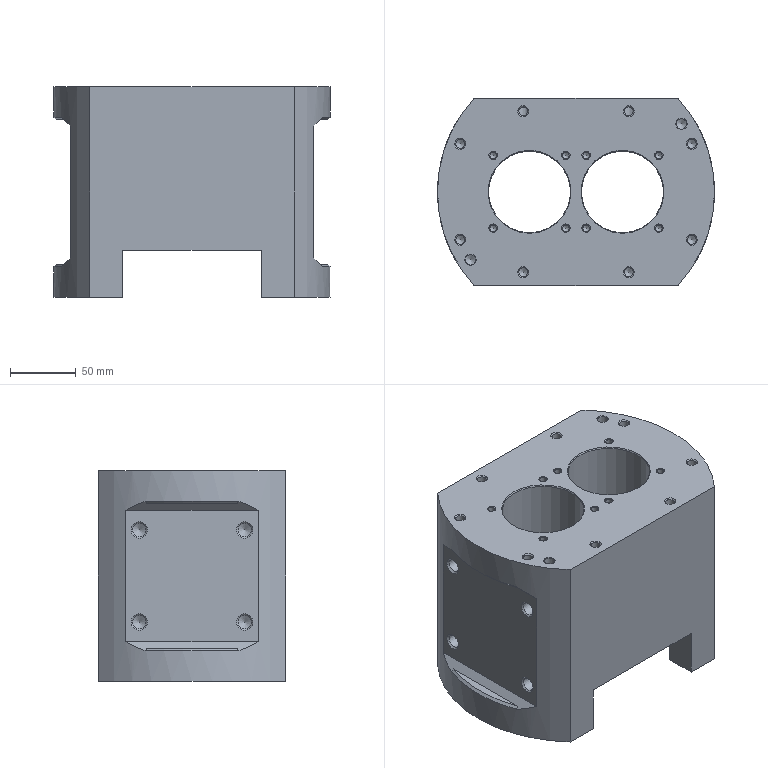NC program | NX | posted with a generic post | part box 210 x 142 x 160 mm
Whole program:
N10 G17 G21 G94 G90
(FLOOR_WALL_COPY_1 , TOOL : D50)
N12 T02 M6
N14 G54
N16 G17 G0 G90 X46.563 Y-89.997 B0. C0. S1200 M3
N18 G43 Z30. H2
N20 Z2.65
N22 G94 G1 Z-0.35 F1000.
N24 X43.563
N26 X-43.563 F2000.
N28 Y-49.998
N30 X43.563
N32 Y-9.999
N34 X-43.563
N36 Y30.001
N38 X43.563
N40 Y70.
N42 X-43.563
N44 X-46.563
N46 Z2.65
N48 G0 Z30.
N50 X50.098 Y-89.997
N52 Z2.301
N54 G1 Z-0.699 F1000.
N56 X47.098
N58 X-47.098 F2000.
N60 Y-49.998
N62 X47.098
N64 Y-9.999
N66 X-47.098
N68 Y30.001
N70 X47.098
N72 Y70.
N74 X-47.098
N76 X-50.098
N78 Z2.301
N80 G0 Z30.
N82 X52.803 Y-89.997
N84 Z1.951
N86 G1 Z-1.049 F1000.
N88 X49.803
N90 X-49.803 F2000.
N92 Y-49.998
N94 X49.803
N96 Y-9.999
N98 X-49.803
N100 Y30.001
N102 X49.803
N104 Y70.
N106 X-49.803
N108 X-52.803
N110 Z1.951
N112 G0 Z30.
N114 X55.078 Y-89.997
N116 Z1.602
N118 G1 Z-1.398 F1000.
N120 X52.078
N122 X-52.078 F2000.
N124 Y-49.998
N126 X52.078
N128 Y-9.999
N130 X-52.078
N132 Y30.001
N134 X52.078
N136 Y70.
N138 X-52.078
N140 X-55.078
N142 Z1.602
N144 G0 Z30.
N146 X57.078 Y-89.997
N148 Z1.252
N150 G1 Z-1.748 F1000.
N152 X54.078
N154 X-54.078 F2000.
N156 Y-49.998
N158 X54.078
N160 Y-9.999
N162 X-54.078
N164 Y30.001
N166 X54.078
N168 Y70.
N170 X-54.078
N172 X-57.078
N174 Z1.252
N176 G0 Z30.
N178 X58.881 Y-89.997
N180 Z0.903
N182 G1 Z-2.097 F1000.
N184 X55.881
N186 X-55.881 F2000.
N188 Y-49.998
N190 X55.881
N192 Y-9.999
N194 X-55.881
N196 Y30.001
N198 X55.881
N200 Y70.
N202 X-55.881
N204 X-58.881
N206 Z0.903
N208 G0 Z30.
N210 X60.535 Y-89.997
N212 Z0.553
N214 G1 Z-2.447 F1000.
N216 X57.535
N218 X-57.535 F2000.
N220 Y-49.998
N222 X57.535
N224 Y-9.999
N226 X-57.535
N228 Y30.001
N230 X57.535
N232 Y70.
N234 X-57.535
N236 X-60.535
N238 Z0.553
N240 G0 Z30.
N242 X62.07 Y-89.997
N244 Z0.204
N246 G1 Z-2.796 F1000.
N248 X59.07
N250 X-59.07 F2000.
N252 Y-49.998
N254 X59.07
N256 Y-9.999
N258 X-59.07
N260 Y30.001
N262 X59.07
N264 Y70.
N266 X-59.07
N268 X-62.07
N270 Z0.204
N272 G0 Z30.
N274 X63.509 Y-89.997
N276 Z-0.146
N278 G1 Z-3.146 F1000.
N280 X60.509
N282 X-60.509 F2000.
N284 Y-49.998
N286 X60.509
N288 Y-9.999
N290 X-60.509
N292 Y30.001
N294 X60.509
N296 Y70.
N298 X-60.509
N300 X-63.509
N302 Z-0.146
N304 G0 Z30.
N306 X64.866 Y-89.997
N308 Z-0.495
N310 G1 Z-3.495 F1000.
N312 X61.866
N314 X-61.866 F2000.
N316 Y-49.998
N318 X61.866
N320 Y-9.999
N322 X-61.866
N324 Y30.001
N326 X61.866
N328 Y70.
N330 X-61.866
N332 X-64.866
N334 Z-0.495
N336 G0 Z30.
N338 X66.153 Y-89.997
N340 Z-0.845
N342 G1 Z-3.845 F1000.
N344 X63.153
N346 X-63.153 F2000.
N348 Y-49.998
N350 X63.153
N352 Y-9.999
N354 X-63.153
N356 Y30.001
N358 X63.153
N360 Y70.
N362 X-63.153
N364 X-66.153
N366 Z-0.845
N368 G0 Z30.
N370 X67.38 Y-89.997
N372 Z-1.194
N374 G1 Z-4.194 F1000.
N376 X64.38
N378 X-64.38 F2000.
N380 Y-49.998
N382 X64.38
N384 Y-9.999
N386 X-64.38
N388 Y30.001
N390 X64.38
N392 Y70.
N394 X-64.38
N396 X-67.38
N398 Z-1.194
N400 G0 Z30.
N402 X68.553 Y-89.997
N404 Z-1.544
N406 G1 Z-4.544 F1000.
N408 X65.553
N410 X-65.553 F2000.
N412 Y-49.998
N414 X65.553
N416 Y-9.999
N418 X-65.553
N420 Y30.001
N422 X65.553
N424 Y70.
N426 X-65.553
N428 X-68.553
N430 Z-1.544
N432 G0 Z30.
N434 X69.68 Y-89.997
N436 Z-1.893
N438 G1 Z-4.893 F1000.
N440 X66.68
N442 X-66.68 F2000.
N444 Y-49.998
N446 X66.68
N448 Y-9.999
N450 X-66.68
N452 Y30.001
N454 X66.68
N456 Y70.
N458 X-66.68
N460 X-69.68
N462 Z-1.893
N464 G0 Z30.
N466 X70.763 Y-89.997
N468 Z-2.243
N470 G1 Z-5.243 F1000.
N472 X67.763
N474 X-67.763 F2000.
N476 Y-49.998
N478 X67.763
N480 Y-9.999
N482 X-67.763
N484 Y30.001
N486 X67.763
N488 Y70.
N490 X-67.763
N492 X-70.763
N494 Z-2.243
N496 G0 Z30.
N498 X71.809 Y-89.997
N500 Z-2.592
N502 G1 Z-5.592 F1000.
N504 X68.809
N506 X-68.809 F2000.
N508 Y-49.998
N510 X68.809
N512 Y-9.999
N514 X-68.809
N516 Y30.001
N518 X68.809
N520 Y70.
N522 X-68.809
N524 X-71.809
N526 Z-2.592
N528 G0 Z30.
N530 X72.82 Y-89.997
N532 Z-2.941
N534 G1 Z-5.941 F1000.
N536 X69.82
N538 X-69.82 F2000.
N540 Y-49.998
N542 X69.82
N544 Y-9.999
N546 X-69.82
N548 Y30.001
N550 X69.82
N552 Y70.
N554 X-69.82
N556 X-72.82
N558 Z-2.941
N560 G0 Z30.
N562 X73.798 Y-89.997
N564 Z-3.291
N566 G1 Z-6.291 F1000.
N568 X70.798
N570 X-70.798 F2000.
N572 Y-49.998
N574 X70.798
N576 Y-9.999
N578 X-70.798
N580 Y30.001
N582 X70.798
N584 Y70.
N586 X-70.798
N588 X-73.798
N590 Z-3.291
N592 G0 Z30.
N594 X74.748 Y-89.997
N596 Z-3.64
N598 G1 Z-6.64 F1000.
N600 X71.748
N602 X-71.748 F2000.
N604 Y-49.998
N606 X71.748
N608 Y-9.999
N610 X-71.748
N612 Y30.001
N614 X71.748
N616 Y70.
N618 X-71.748
N620 X-74.748
N622 Z-3.64
N624 G0 Z30.
N626 X75.67 Y-89.997
N628 Z-3.99
N630 G1 Z-6.99 F1000.
N632 X72.67
N634 X-72.67 F2000.
N636 Y-49.998
N638 X72.67
N640 Y-9.999
N642 X-72.67
N644 Y30.001
N646 X72.67
N648 Y70.
N650 X-72.67
N652 X-75.67
N654 Z-3.99
N656 G0 Z30.
N658 X76.567 Y-89.997
N660 Z-4.339
N662 G1 Z-7.339 F1000.
N664 X73.567
N666 X-73.567 F2000.
N668 Y-49.998
N670 X73.567
N672 Y-9.999
N674 X-73.567
N676 Y30.001
N678 X73.567
N680 Y70.
N682 X-73.567
N684 X-76.567
N686 Z-4.339
N688 G0 Z30.
N690 X77.44 Y-89.997
N692 Z-4.689
N694 G1 Z-7.689 F1000.
N696 X74.44
N698 X-74.44 F2000.
N700 Y-49.998
N702 X74.44
N704 Y-9.999
N706 X-74.44
N708 Y30.001
N710 X74.44
N712 Y70.
N714 X-74.44
N716 X-77.44
N718 Z-4.689
N720 G0 Z30.
N722 X78.292 Y-89.997
N724 Z-5.038
N726 G1 Z-8.038 F1000.
N728 X75.292
N730 X-75.292 F2000.
N732 Y-49.998
N734 X75.292
N736 Y-9.999
N738 X-75.292
N740 Y30.001
N742 X75.292
N744 Y70.
N746 X-75.292
N748 X-78.292
N750 Z-5.038
N752 G0 Z30.
N754 X79.123 Y-89.997
N756 Z-5.388
N758 G1 Z-8.388 F1000.
N760 X76.123
N762 X-76.123 F2000.
N764 Y-49.998
N766 X76.123
N768 Y-9.999
N770 X-76.123
N772 Y30.001
N774 X76.123
N776 Y70.
N778 X-76.123
N780 X-79.123
N782 Z-5.388
N784 G0 Z30.
N786 X79.934 Y-89.997
N788 Z-5.737
N790 G1 Z-8.737 F1000.
N792 X76.934
N794 X-76.934 F2000.
N796 Y-49.998
N798 X76.934
N800 Y-9.999
N802 X-76.934
N804 Y30.001
N806 X76.934
N808 Y70.
N810 X-76.934
N812 X-79.934
N814 Z-5.737
N816 G0 Z30.
N818 X80.728 Y-89.997
N820 Z-6.087
N822 G1 Z-9.087 F1000.
N824 X77.728
N826 X-77.728 F2000.
N828 Y-49.998
N830 X77.728
N832 Y-9.999
N834 X-77.728
N836 Y30.001
N838 X77.728
N840 Y70.
N842 X-77.728
N844 X-80.728
N846 Z-6.087
N848 G0 Z30.
N850 X81.504 Y-89.997
N852 Z-6.436
N854 G1 Z-9.436 F1000.
N856 X78.504
N858 X-78.504 F2000.
N860 Y-49.998
N862 X78.504
N864 Y-9.999
N866 X-78.504
N868 Y30.001
N870 X78.504
N872 Y70.
N874 X-78.504
N876 X-81.504
N878 Z-6.436
N880 G0 Z30.
N882 X82.263 Y-89.997
N884 Z-6.786
N886 G1 Z-9.786 F1000.
N888 X79.263
N890 X-79.263 F2000.
N892 Y-49.998
N894 X79.263
N896 Y-9.999
N898 X-79.263
N900 Y30.001
N902 X79.263
N904 Y70.
N906 X-79.263
N908 X-82.263
N910 Z-6.786
N912 G0 Z30.
N914 X83.008 Y-89.997
N916 Z-7.135
N918 G1 Z-10.135 F1000.
N920 X80.008
N922 X-80.008 F2000.
N924 Y-49.998
N926 X80.008
N928 Y-9.999
N930 X-80.008
N932 Y30.001
N934 X80.008
N936 Y70.
N938 X-80.008
N940 X-83.008
N942 Z-7.135
N944 G0 Z30.
N946 X83.737 Y-89.997
N948 Z-7.485
N950 G1 Z-10.485 F1000.
N952 X80.737
N954 X-80.737 F2000.
N956 Y-49.998
N958 X80.737
N960 Y-9.999
N962 X-80.737
N964 Y30.001
N966 X80.737
N968 Y70.
N970 X-80.737
N972 X-83.737
N974 Z-7.485
N976 G0 Z30.
N978 X84.452 Y-89.997
N980 Z-7.834
N982 G1 Z-10.834 F1000.
N984 X81.452
N986 X-81.452 F2000.
N988 Y-49.998
N990 X81.452
N992 Y-9.999
N994 X-81.452
N996 Y30.001
N998 X81.452
N1000 Y70.
N1002 X-81.452
N1004 X-84.452
N1006 Z-7.834
N1008 G0 Z30.
N1010 X85.154 Y-89.997
N1012 Z-8.184
N1014 G1 Z-11.184 F1000.
N1016 X82.154
N1018 X-82.154 F2000.
N1020 Y-49.998
N1022 X82.154
N1024 Y-9.999
N1026 X-82.154
N1028 Y30.001
N1030 X82.154
N1032 Y70.
N1034 X-82.154
N1036 X-85.154
N1038 Z-8.184
N1040 G0 Z30.
N1042 X85.843 Y-89.997
N1044 Z-8.533
N1046 G1 Z-11.533 F1000.
N1048 X82.843
N1050 X-82.843 F2000.
N1052 Y-49.998
N1054 X82.843
N1056 Y-9.999
N1058 X-82.843
N1060 Y30.001
N1062 X82.843
N1064 Y70.
N1066 X-82.843
N1068 X-85.843
N1070 Z-8.533
N1072 G0 Z30.
N1074 X86.52 Y-89.997
N1076 Z-8.883
N1078 G1 Z-11.883 F1000.
N1080 X83.52
N1082 X-83.52 F2000.
N1084 Y-49.998
N1086 X83.52
N1088 Y-9.999
N1090 X-83.52
N1092 Y30.001
N1094 X83.52
N1096 Y70.
N1098 X-83.52
N1100 X-86.52
N1102 Z-8.883
N1104 G0 Z30.
N1106 X87.185 Y-89.997
N1108 Z-9.232
N1110 G1 Z-12.232 F1000.
N1112 X84.185
N1114 X-84.185 F2000.
N1116 Y-49.998
N1118 X84.185
N1120 Y-9.999
N1122 X-84.185
N1124 Y30.001
N1126 X84.185
N1128 Y70.
N1130 X-84.185
N1132 X-87.185
N1134 Z-9.232
N1136 G0 Z30.
N1138 X87.838 Y-89.997
N1140 Z-9.582
N1142 G1 Z-12.582 F1000.
N1144 X84.838
N1146 X-84.838 F2000.
N1148 Y-49.998
N1150 X84.838
N1152 Y-9.999
N1154 X-84.838
N1156 Y30.001
N1158 X84.838
N1160 Y70.
N1162 X-84.838
N1164 X-87.838
N1166 Z-9.582
N1168 G0 Z30.
N1170 X88.481 Y-89.997
N1172 Z-9.931
N1174 G1 Z-12.931 F1000.
N1176 X85.481
N1178 X-85.481 F2000.
N1180 Y-49.998
N1182 X85.481
N1184 Y-9.999
N1186 X-85.481
N1188 Y30.001
N1190 X85.481
N1192 Y70.
N1194 X-85.481
N1196 X-88.481
N1198 Z-9.931
N1200 G0 Z30.
N1202 X89.113 Y-89.997
N1204 Z-10.281
N1206 G1 Z-13.281 F1000.
N1208 X86.113
N1210 X-86.113 F2000.
N1212 Y-49.998
N1214 X86.113
N1216 Y-9.999
N1218 X-86.113
N1220 Y30.001
N1222 X86.113
N1224 Y70.
N1226 X-86.113
N1228 X-89.113
N1230 Z-10.281
N1232 G0 Z30.
N1234 X89.735 Y-89.997
N1236 Z-10.63
N1238 G1 Z-13.63 F1000.
N1240 X86.735
N1242 X-86.735 F2000.
N1244 Y-49.998
N1246 X86.735
N1248 Y-9.999
N1250 X-86.735
N1252 Y30.001
N1254 X86.735
N1256 Y70.
N1258 X-86.735
N1260 X-89.735
N1262 Z-10.63
N1264 G0 Z30.
N1266 X90.348 Y-89.997
N1268 Z-10.98
N1270 G1 Z-13.98 F1000.
N1272 X87.348
N1274 X-87.348 F2000.
N1276 Y-49.998
N1278 X87.348
N1280 Y-9.999
N1282 X-87.348
N1284 Y30.001
N1286 X87.348
N1288 Y70.
N1290 X-87.348
N1292 X-90.348
N1294 Z-10.98
N1296 G0 Z30.
N1298 X90.951 Y-89.997
N1300 Z-11.329
N1302 G1 Z-14.329 F1000.
N1304 X87.951
N1306 X-87.951 F2000.
N1308 Y-49.998
N1310 X87.951
N1312 Y-9.999
N1314 X-87.951
N1316 Y30.001
N1318 X87.951
N1320 Y70.
N1322 X-87.951
N1324 X-90.951
N1326 Z-11.329
N1328 G0 Z30.
N1330 X91.545 Y-89.997
N1332 Z-11.679
N1334 G1 Z-14.679 F1000.
N1336 X88.545
N1338 X-88.545 F2000.
N1340 Y-49.998
N1342 X88.545
N1344 Y-9.999
N1346 X-88.545
N1348 Y30.001
N1350 X88.545
N1352 Y70.
N1354 X-88.545
N1356 X-91.545
N1358 Z-11.679
N1360 G0 Z30.
N1362 X92.13 Y-89.997
N1364 Z-12.028
N1366 G1 Z-15.028 F1000.
N1368 X89.13
N1370 X-89.13 F2000.
N1372 Y-49.998
N1374 X89.13
N1376 Y-9.999
N1378 X-89.13
N1380 Y30.001
N1382 X89.13
N1384 Y70.
N1386 X-89.13
N1388 X-92.13
N1390 Z-12.028
N1392 G0 Z30.
N1394 X92.707 Y-89.997
N1396 Z-12.377
N1398 G1 Z-15.377 F1000.
N1400 X89.707
N1402 X-89.707 F2000.
N1404 Y-49.998
N1406 X89.707
N1408 Y-9.999
N1410 X-89.707
N1412 Y30.001
N1414 X89.707
N1416 Y70.
N1418 X-89.707
N1420 X-92.707
N1422 Z-12.377
N1424 G0 Z30.
N1426 X93.275 Y-89.997
N1428 Z-12.727
N1430 G1 Z-15.727 F1000.
N1432 X90.275
N1434 X-90.275 F2000.
N1436 Y-49.998
N1438 X90.275
N1440 Y-9.999
N1442 X-90.275
N1444 Y30.001
N1446 X90.275
N1448 Y70.
N1450 X-90.275
N1452 X-93.275
N1454 Z-12.727
N1456 G0 Z30.
N1458 X93.835 Y-89.997
N1460 Z-13.076
N1462 G1 Z-16.076 F1000.
N1464 X90.835
N1466 X-90.835 F2000.
N1468 Y-49.998
N1470 X90.835
N1472 Y-9.999
N1474 X-90.835
N1476 Y30.001
N1478 X90.835
N1480 Y70.
N1482 X-90.835
N1484 X-93.835
N1486 Z-13.076
N1488 G0 Z30.
N1490 X94.388 Y-89.997
N1492 Z-13.426
N1494 G1 Z-16.426 F1000.
N1496 X91.388
N1498 X-91.388 F2000.
N1500 Y-49.998
N1502 X91.388
N1504 Y-9.999
N1506 X-91.388
N1508 Y30.001
N1510 X91.388
N1512 Y70.
N1514 X-91.388
N1516 X-94.388
N1518 Z-13.426
N1520 G0 Z30.
N1522 X94.933 Y-89.997
N1524 Z-13.775
N1526 G1 Z-16.775 F1000.
N1528 X91.933
N1530 X-91.933 F2000.
N1532 Y-49.998
N1534 X91.933
N1536 Y-9.999
N1538 X-91.933
N1540 Y30.001
N1542 X91.933
N1544 Y70.
N1546 X-91.933
N1548 X-94.933
N1550 Z-13.775
N1552 G0 Z30.
N1554 X95.471 Y-89.997
N1556 Z-14.125
N1558 G1 Z-17.125 F1000.
N1560 X92.471
N1562 X-92.471 F2000.
N1564 Y-49.998
N1566 X92.471
N1568 Y-9.999
N1570 X-92.471
N1572 Y30.001
N1574 X92.471
N1576 Y70.
N1578 X-92.471
N1580 X-95.471
N1582 Z-14.125
N1584 G0 Z30.
N1586 X96.002 Y-89.997
N1588 Z-14.474
N1590 G1 Z-17.474 F1000.
N1592 X93.002
N1594 X-93.002 F2000.
N1596 Y-49.998
N1598 X93.002
N1600 Y-9.999
N1602 X-93.002
N1604 Y30.001
N1606 X93.002
N1608 Y70.
N1610 X-93.002
N1612 X-96.002
N1614 Z-14.474
N1616 G0 Z30.
N1618 X96.526 Y-89.997
N1620 Z-14.824
N1622 G1 Z-17.824 F1000.
N1624 X93.526
N1626 X-93.526 F2000.
N1628 Y-49.998
N1630 X93.526
N1632 Y-9.999
N1634 X-93.526
N1636 Y30.001
N1638 X93.526
N1640 Y70.
N1642 X-93.526
N1644 X-96.526
N1646 Z-14.824
N1648 G0 Z30.
N1650 X97.043 Y-89.997
N1652 Z-15.173
N1654 G1 Z-18.173 F1000.
N1656 X94.043
N1658 X-94.043 F2000.
N1660 Y-49.998
N1662 X94.043
N1664 Y-9.999
N1666 X-94.043
N1668 Y30.001
N1670 X94.043
N1672 Y70.
N1674 X-94.043
N1676 X-97.043
N1678 Z-15.173
N1680 G0 Z30.
N1682 X97.554 Y-89.997
N1684 Z-15.523
N1686 G1 Z-18.523 F1000.
N1688 X94.554
N1690 X-94.554 F2000.
N1692 Y-49.998
N1694 X94.554
N1696 Y-9.999
N1698 X-94.554
N1700 Y30.001
N1702 X94.554
N1704 Y70.
N1706 X-94.554
N1708 X-97.554
N1710 Z-15.523
N1712 G0 Z30.
N1714 X98.058 Y-89.997
N1716 Z-15.872
N1718 G1 Z-18.872 F1000.
N1720 X95.058
N1722 X-95.058 F2000.
N1724 Y-49.998
N1726 X95.058
N1728 Y-9.999
N1730 X-95.058
N1732 Y30.001
N1734 X95.058
N1736 Y70.
N1738 X-95.058
N1740 X-98.058
N1742 Z-15.872
N1744 G0 Z30.
N1746 X98.557 Y-89.997
N1748 Z-16.222
N1750 G1 Z-19.222 F1000.
N1752 X95.557
N1754 X-95.557 F2000.
N1756 Y-49.998
N1758 X95.557
N1760 Y-9.999
N1762 X-95.557
N1764 Y30.001
N1766 X95.557
N1768 Y70.
N1770 X-95.557
N1772 X-98.557
N1774 Z-16.222
N1776 G0 Z30.
N1778 X99.049 Y-89.997
N1780 Z-16.571
N1782 G1 Z-19.571 F1000.
N1784 X96.049
N1786 X-96.049 F2000.
N1788 Y-49.998
N1790 X96.049
N1792 Y-9.999
N1794 X-96.049
N1796 Y30.001
N1798 X96.049
N1800 Y70.
N1802 X-96.049
N1804 X-99.049
N1806 Z-16.571
N1808 G0 Z30.
N1810 X99.535 Y-89.997
N1812 Z-16.921
N1814 G1 Z-19.921 F1000.
N1816 X96.535
N1818 X-96.535 F2000.
N1820 Y-49.998
N1822 X96.535
N1824 Y-9.999
N1826 X-96.535
N1828 Y30.001
N1830 X96.535
N1832 Y70.
N1834 X-96.535
N1836 X-99.535
N1838 Z-16.921
N1840 G0 Z30.
N1842 X100.015 Y-89.997
N1844 Z-17.27
N1846 G1 Z-20.27 F1000.
N1848 X97.015
N1850 X-97.015 F2000.
N1852 Y-49.998
N1854 X97.015
N1856 Y-9.999
N1858 X-97.015
N1860 Y30.001
N1862 X97.015
N1864 Y70.
N1866 X-97.015
N1868 X-100.015
N1870 Z-17.27
N1872 G0 Z30.
N1874 X100.49 Y-89.997
N1876 Z-17.62
N1878 G1 Z-20.62 F1000.
N1880 X97.49
N1882 X-97.49 F2000.
N1884 Y-49.998
N1886 X97.49
N1888 Y-9.999
N1890 X-97.49
N1892 Y30.001
N1894 X97.49
N1896 Y70.
N1898 X-97.49
N1900 X-100.49
N1902 Z-17.62
N1904 G0 Z30.
N1906 X100.959 Y-89.997
N1908 Z-17.969
N1910 G1 Z-20.969 F1000.
N1912 X97.959
N1914 X-97.959 F2000.
N1916 Y-49.998
N1918 X97.959
N1920 Y-9.999
N1922 X-97.959
N1924 Y30.001
N1926 X97.959
N1928 Y70.
N1930 X-97.959
N1932 X-100.959
N1934 Z-17.969
N1936 G0 Z30.
N1938 X101.423 Y-89.997
N1940 Z-18.319
N1942 G1 Z-21.319 F1000.
N1944 X98.423
N1946 X-98.423 F2000.
N1948 Y-49.998
N1950 X98.423
N1952 Y-9.999
N1954 X-98.423
N1956 Y30.001
N1958 X98.423
N1960 Y70.
N1962 X-98.423
N1964 X-101.423
N1966 Z-18.319
N1968 G0 Z30.
N1970 X101.881 Y-89.997
N1972 Z-18.668
N1974 G1 Z-21.668 F1000.
N1976 X98.881
N1978 X-98.881 F2000.
N1980 Y-49.998
N1982 X98.881
N1984 Y-9.999
N1986 X-98.881
N1988 Y30.001
N1990 X98.881
N1992 Y70.
N1994 X-98.881
N1996 X-101.881
N1998 Z-18.668
N2000 G0 Z30.
N2002 X102.334 Y-89.997
N2004 Z-19.018
N2006 G1 Z-22.018 F1000.
N2008 X99.334
N2010 X-99.334 F2000.
N2012 Y-49.998
N2014 X99.334
N2016 Y-9.999
N2018 X-99.334
N2020 Y30.001
N2022 X99.334
N2024 Y70.
N2026 X-99.334
N2028 X-102.334
N2030 Z-19.018
N2032 G0 Z30.
N2034 X102.783 Y-89.997
N2036 Z-19.367
N2038 G1 Z-22.367 F1000.
N2040 X99.783
N2042 X-99.783 F2000.
N2044 Y-49.998
N2046 X99.783
N2048 Y-9.999
N2050 X-99.783
N2052 Y30.001
N2054 X99.783
N2056 Y70.
N2058 X-99.783
N2060 X-102.783
N2062 Z-19.367
N2064 G0 Z30.
N2066 X103.226 Y-89.997
N2068 Z-19.717
N2070 G1 Z-22.717 F1000.
N2072 X100.226
N2074 X-100.226 F2000.
N2076 Y-49.998
N2078 X100.226
N2080 Y-9.999
N2082 X-100.226
N2084 Y30.001
N2086 X100.226
N2088 Y70.
N2090 X-100.226
N2092 X-103.226
N2094 Z-19.717
N2096 G0 Z30.
N2098 X103.665 Y-89.997
N2100 Z-20.066
N2102 G1 Z-23.066 F1000.
N2104 X100.665
N2106 X-100.665 F2000.
N2108 Y-49.998
N2110 X100.665
N2112 Y-9.999
N2114 X-100.665
N2116 Y30.001
N2118 X100.665
N2120 Y70.
N2122 X-100.665
N2124 X-103.665
N2126 Z-20.066
N2128 G0 Z30.
N2130 X104.098 Y-89.997
N2132 Z-20.416
N2134 G1 Z-23.416 F1000.
N2136 X101.098
N2138 X-101.098 F2000.
N2140 Y-49.998
N2142 X101.098
N2144 Y-9.999
N2146 X-101.098
N2148 Y30.001
N2150 X101.098
N2152 Y70.
N2154 X-101.098
N2156 X-104.098
N2158 Z-20.416
N2160 G0 Z30.
N2162 X104.527 Y-89.997
N2164 Z-20.765
N2166 G1 Z-23.765 F1000.
N2168 X101.527
N2170 X-101.527 F2000.
N2172 Y-49.998
N2174 X101.527
N2176 Y-9.999
N2178 X-101.527
N2180 Y30.001
N2182 X101.527
N2184 Y70.
N2186 X-101.527
N2188 X-104.527
N2190 Z-20.765
N2192 G0 Z30.
N2194 X104.952 Y-89.997
N2196 Z-21.115
N2198 G1 Z-24.115 F1000.
N2200 X101.952
N2202 X-101.952 F2000.
N2204 Y-49.998
N2206 X101.952
N2208 Y-9.999
N2210 X-101.952
N2212 Y30.001
N2214 X101.952
N2216 Y70.
N2218 X-101.952
N2220 X-104.952
N2222 Z-21.115
N2224 G0 Z30.
N2226 X105.372 Y-89.997
N2228 Z-21.464
N2230 G1 Z-24.464 F1000.
N2232 X102.372
N2234 X-102.372 F2000.
N2236 Y-49.998
N2238 X102.372
N2240 Y-9.999
N2242 X-102.372
N2244 Y30.001
N2246 X102.372
N2248 Y70.
N2250 X-102.372
N2252 X-105.372
N2254 Z-21.464
N2256 G0 Z30.
N2258 X105.787 Y-89.997
N2260 Z-21.813
N2262 G1 Z-24.813 F1000.
N2264 X102.787
N2266 X-102.787 F2000.
N2268 Y-49.998
N2270 X102.787
N2272 Y-9.999
N2274 X-102.787
N2276 Y30.001
N2278 X102.787
N2280 Y70.
N2282 X-102.787
N2284 X-105.787
N2286 Z-21.813
N2288 G0 Z30.
N2290 X106.199 Y-89.997
N2292 Z-22.163
N2294 G1 Z-25.163 F1000.
N2296 X103.199
N2298 X-103.199 F2000.
N2300 Y-49.998
N2302 X103.199
N2304 Y-9.999
N2306 X-103.199
N2308 Y30.001
N2310 X103.199
N2312 Y70.
N2314 X-103.199
N2316 X-106.199
N2318 Z-22.163
N2320 G0 Z30.
N2322 X106.606 Y-89.997
N2324 Z-22.512
N2326 G1 Z-25.512 F1000.
N2328 X103.606
N2330 X-103.606 F2000.
N2332 Y-49.998
N2334 X103.606
N2336 Y-9.999
N2338 X-103.606
N2340 Y30.001
N2342 X103.606
N2344 Y70.
N2346 X-103.606
N2348 X-106.606
N2350 Z-22.512
N2352 G0 Z30.
N2354 X107.008 Y-89.997
N2356 Z-22.862
N2358 G1 Z-25.862 F1000.
N2360 X104.008
N2362 X-104.008 F2000.
N2364 Y-49.998
N2366 X104.008
N2368 Y-9.999
N2370 X-104.008
N2372 Y30.001
N2374 X104.008
N2376 Y70.
N2378 X-104.008
N2380 X-107.008
N2382 Z-22.862
N2384 G0 Z30.
N2386 X107.407 Y-89.997
N2388 Z-23.211
N2390 G1 Z-26.211 F1000.
N2392 X104.407
N2394 X-104.407 F2000.
N2396 Y-49.998
N2398 X104.407
N2400 Y-9.999
N2402 X-104.407
N2404 Y30.001
N2406 X104.407
N2408 Y70.
N2410 X-104.407
N2412 X-107.407
N2414 Z-23.211
N2416 G0 Z30.
N2418 X107.802 Y-89.997
N2420 Z-23.561
N2422 G1 Z-26.561 F1000.
N2424 X104.802
N2426 X-104.802 F2000.
N2428 Y-49.998
N2430 X104.802
N2432 Y-9.999
N2434 X-104.802
N2436 Y30.001
N2438 X104.802
N2440 Y70.
N2442 X-104.802
N2444 X-107.802
N2446 Z-23.561
N2448 G0 Z30.
N2450 X108.193 Y-89.997
N2452 Z-23.91
N2454 G1 Z-26.91 F1000.
N2456 X105.193
N2458 X-105.193 F2000.
N2460 Y-49.998
N2462 X105.193
N2464 Y-9.999
N2466 X-105.193
N2468 Y30.001
N2470 X105.193
N2472 Y70.
N2474 X-105.193
N2476 X-108.193
N2478 Z-23.91
N2480 G0 Z30.
N2482 X108.58 Y-89.997
N2484 Z-24.26
N2486 G1 Z-27.26 F1000.
N2488 X105.58
N2490 X-105.58 F2000.
N2492 Y-49.998
N2494 X105.58
N2496 Y-9.999
N2498 X-105.58
N2500 Y30.001
N2502 X105.58
N2504 Y70.
N2506 X-105.58
N2508 X-108.58
N2510 Z-24.26
N2512 G0 Z30.
N2514 X108.963 Y-89.997
N2516 Z-24.609
N2518 G1 Z-27.609 F1000.
N2520 X105.963
N2522 X-105.963 F2000.
N2524 Y-49.998
N2526 X105.963
N2528 Y-9.999
N2530 X-105.963
N2532 Y30.001
N2534 X105.963
N2536 Y70.
N2538 X-105.963
N2540 X-108.963
N2542 Z-24.609
N2544 G0 Z30.
N2546 X109.342 Y-89.997
N2548 Z-24.959
N2550 G1 Z-27.959 F1000.
N2552 X106.342
N2554 X-106.342 F2000.
N2556 Y-49.998
N2558 X106.342
N2560 Y-9.999
N2562 X-106.342
N2564 Y30.001
N2566 X106.342
N2568 Y70.
N2570 X-106.342
N2572 X-109.342
N2574 Z-24.959
N2576 G0 Z30.
N2578 X109.717 Y-89.997
N2580 Z-25.308
N2582 G1 Z-28.308 F1000.
N2584 X106.717
N2586 X-106.717 F2000.
N2588 Y-49.998
N2590 X106.717
N2592 Y-9.999
N2594 X-106.717
N2596 Y30.001
N2598 X106.717
N2600 Y70.
N2602 X-106.717
N2604 X-109.717
N2606 Z-25.308
N2608 G0 Z30.
N2610 X110.089 Y-89.997
N2612 Z-25.658
N2614 G1 Z-28.658 F1000.
N2616 X107.089
N2618 X-107.089 F2000.
N2620 Y-49.998
N2622 X107.089
N2624 Y-9.999
N2626 X-107.089
N2628 Y30.001
N2630 X107.089
N2632 Y70.
N2634 X-107.089
N2636 X-110.089
N2638 Z-25.658
N2640 G0 Z30.
N2642 X110.458 Y-89.997
N2644 Z-26.007
N2646 G1 Z-29.007 F1000.
N2648 X107.458
N2650 X-107.458 F2000.
N2652 Y-49.998
N2654 X107.458
N2656 Y-9.999
N2658 X-107.458
N2660 Y30.001
N2662 X107.458
N2664 Y70.
N2666 X-107.458
N2668 X-110.458
N2670 Z-26.007
N2672 G0 Z30.
N2674 X110.822 Y-89.997
N2676 Z-26.357
N2678 G1 Z-29.357 F1000.
N2680 X107.822
N2682 X-107.822 F2000.
N2684 Y-49.998
N2686 X107.822
N2688 Y-9.999
N2690 X-107.822
N2692 Y30.001
N2694 X107.822
N2696 Y70.
N2698 X-107.822
N2700 X-110.822
N2702 Z-26.357
N2704 G0 Z30.
N2706 X111.184 Y-89.997
N2708 Z-26.706
N2710 G1 Z-29.706 F1000.
N2712 X108.184
N2714 X-108.184 F2000.
N2716 Y-49.998
N2718 X108.184
N2720 Y-9.999
N2722 X-108.184
N2724 Y30.001
N2726 X108.184
N2728 Y70.
N2730 X-108.184
N2732 X-111.184
N2734 Z-26.706
N2736 G0 Z30.
N2738 X111.542 Y-89.997
N2740 Z-27.056
N2742 G1 Z-30.056 F1000.
N2744 X108.542
N2746 X-108.542 F2000.
N2748 Y-49.998
N2750 X108.542
N2752 Y-9.999
N2754 X-108.542
N2756 Y30.001
N2758 X108.542
N2760 Y70.
N2762 X-108.542
N2764 X-111.542
N2766 Z-27.056
N2768 G0 Z30.
N2770 X111.896 Y-89.997
N2772 Z-27.405
N2774 G1 Z-30.405 F1000.
N2776 X108.896
N2778 X-108.896 F2000.
N2780 Y-49.998
N2782 X108.896
N2784 Y-9.999
N2786 X-108.896
N2788 Y30.001
N2790 X108.896
N2792 Y70.
N2794 X-108.896
N2796 X-111.896
N2798 Z-27.405
N2800 G0 Z30.
N2802 X112.247 Y-89.997
N2804 Z-27.755
N2806 G1 Z-30.755 F1000.
N2808 X109.247
N2810 X-109.247 F2000.
N2812 Y-49.998
N2814 X109.247
N2816 Y-9.999
N2818 X-109.247
N2820 Y30.001
N2822 X109.247
N2824 Y70.
N2826 X-109.247
N2828 X-112.247
N2830 Z-27.755
N2832 G0 Z30.
N2834 X112.595 Y-89.997
N2836 Z-28.104
N2838 G1 Z-31.104 F1000.
N2840 X109.595
N2842 X-109.595 F2000.
N2844 Y-49.998
N2846 X109.595
N2848 Y-9.999
N2850 X-109.595
N2852 Y30.001
N2854 X109.595
N2856 Y70.
N2858 X-109.595
N2860 X-112.595
N2862 Z-28.104
N2864 G0 Z30.
N2866 X112.94 Y-89.997
N2868 Z-28.454
N2870 G1 Z-31.454 F1000.
N2872 X109.94
N2874 X-109.94 F2000.
N2876 Y-49.998
N2878 X109.94
N2880 Y-9.999
N2882 X-109.94
N2884 Y30.001
N2886 X109.94
N2888 Y70.
N2890 X-109.94
N2892 X-112.94
N2894 Z-28.454
N2896 G0 Z30.
N2898 X113.281 Y-89.997
N2900 Z-28.803
N2902 G1 Z-31.803 F1000.
N2904 X110.281
N2906 X-110.281 F2000.
N2908 Y-49.998
N2910 X110.281
N2912 Y-9.999
N2914 X-110.281
N2916 Y30.001
N2918 X110.281
N2920 Y70.
N2922 X-110.281
N2924 X-113.281
N2926 Z-28.803
N2928 G0 Z30.
N2930 X113.619 Y-89.997
N2932 Z-29.153
N2934 G1 Z-32.153 F1000.
N2936 X110.619
N2938 X-110.619 F2000.
N2940 Y-49.998
N2942 X110.619
N2944 Y-9.999
N2946 X-110.619
N2948 Y30.001
N2950 X110.619
N2952 Y70.
N2954 X-110.619
N2956 X-113.619
N2958 Z-29.153
N2960 G0 Z30.
N2962 X113.954 Y-89.997
N2964 Z-29.502
N2966 G1 Z-32.502 F1000.
N2968 X110.954
N2970 X-110.954 F2000.
N2972 Y-49.998
N2974 X110.954
N2976 Y-9.999
N2978 X-110.954
N2980 Y30.001
N2982 X110.954
N2984 Y70.
N2986 X-110.954
N2988 X-113.954
N2990 Z-29.502
N2992 G0 Z30.
N2994 X114.286 Y-89.997
N2996 Z-29.852
N2998 G1 Z-32.852 F1000.
N3000 X111.286
N3002 X-111.286 F2000.
N3004 Y-49.998
N3006 X111.286
N3008 Y-9.999
N3010 X-111.286
N3012 Y30.001
N3014 X111.286
N3016 Y70.
N3018 X-111.286
N3020 X-114.286
N3022 Z-29.852
N3024 G0 Z30.
N3026 X114.615 Y-89.997
N3028 Z-30.201
N3030 G1 Z-33.201 F1000.
N3032 X111.615
N3034 X-111.615 F2000.
N3036 Y-49.998
N3038 X111.615
N3040 Y-9.999
N3042 X-111.615
N3044 Y30.001
N3046 X111.615
N3048 Y70.
N3050 X-111.615
N3052 X-114.615
N3054 Z-30.201
N3056 G0 Z30.
N3058 X114.941 Y-89.997
N3060 Z-30.551
N3062 G1 Z-33.551 F1000.
N3064 X111.941
N3066 X-111.941 F2000.
N3068 Y-49.998
N3070 X111.941
N3072 Y-9.999
N3074 X-111.941
N3076 Y30.001
N3078 X111.941
N3080 Y70.
N3082 X-111.941
N3084 X-114.941
N3086 Z-30.551
N3088 G0 Z30.
N3090 X115.264 Y-89.997
N3092 Z-30.9
N3094 G1 Z-33.9 F1000.
N3096 X112.264
N3098 X-112.264 F2000.
N3100 Y-49.998
N3102 X112.264
N3104 Y-9.999
N3106 X-112.264
N3108 Y30.001
N3110 X112.264
N3112 Y70.
N3114 X-112.264
N3116 X-115.264
N3118 Z-30.9
N3120 G0 Z30.
(FLOOR_WALL_COPY_COPY , TOOL : D50)
N3122 X115.356 Y-89.997 S2500
N3124 Z-31.
N3126 G1 Z-34. F1000.
N3128 X112.356
N3130 X-112.356
N3132 Y-49.998
N3134 X112.356
N3136 Y-9.999
N3138 X-112.356
N3140 Y30.001
N3142 X112.356
N3144 Y70.
N3146 X-112.356
N3148 X-115.356
N3150 Z-31.
N3152 G0 Z30.
N3154 M5
N3156 M2